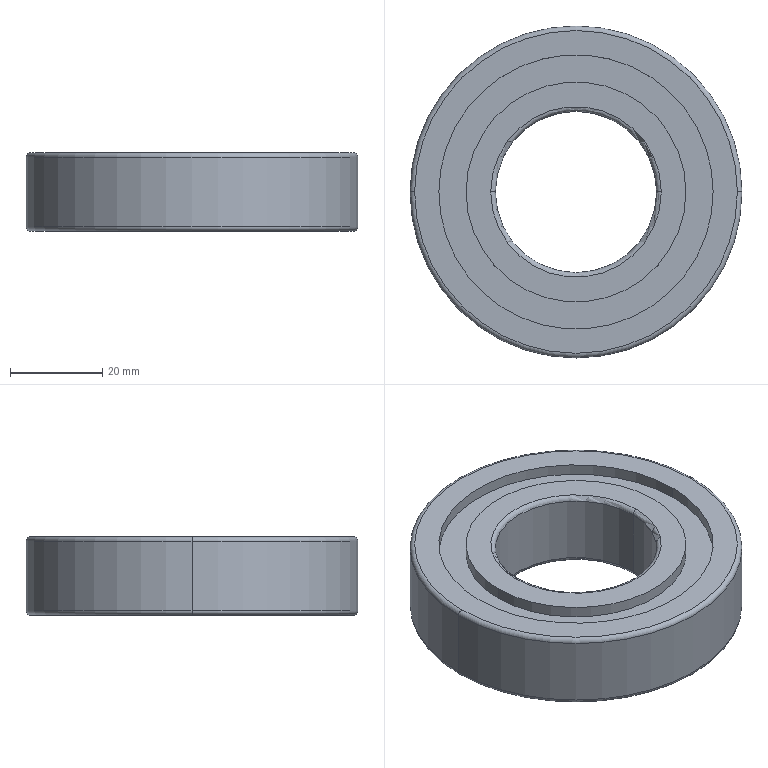Part | SolidWorks | features BaseBody 1 | 1 solid | 26 faces | box 72 x 72 x 17 mm | volume 47748 mm3 | cylinder 12 | torus 8 | plane 6 | commonest cylinder face diameters 47.7 x4 59.5 x4 35 x2 72 x2
STEP:
#1=CARTESIAN_POINT('',(358.083,269.388,35.922));
#2=VERTEX_POINT('',#1);
#3=CARTESIAN_POINT('',(323.083,269.388,35.922));
#4=VERTEX_POINT('',#3);
#5=CARTESIAN_POINT('',(340.583,269.388,35.922));
#6=DIRECTION('',(0.,0.,1.));
#7=DIRECTION('',(-1.,-0.000000008,0.));
#8=AXIS2_PLACEMENT_3D('',#5,#6,#7);
#9=CIRCLE('',#8,17.5);
#10=EDGE_CURVE('',#2,#4,#9,.T.);
#11=ORIENTED_EDGE('',*,*,#10,.T.);
#12=CARTESIAN_POINT('',(322.083,269.388,34.922));
#13=VERTEX_POINT('',#12);
#14=CARTESIAN_POINT('',(322.083,269.388,35.922));
#15=DIRECTION('',(-0.000000008,1.,0.));
#16=DIRECTION('',(-1.,-0.000000008,0.));
#17=AXIS2_PLACEMENT_3D('',#14,#15,#16);
#18=CIRCLE('',#17,1.);
#19=EDGE_CURVE('',#4,#13,#18,.T.);
#20=ORIENTED_EDGE('',*,*,#19,.T.);
#21=CARTESIAN_POINT('',(359.083,269.388,34.922));
#22=VERTEX_POINT('',#21);
#23=CARTESIAN_POINT('',(340.583,269.388,34.922));
#24=DIRECTION('',(0.,0.,1.));
#25=DIRECTION('',(-1.,-0.000000008,0.));
#26=AXIS2_PLACEMENT_3D('',#23,#24,#25);
#27=CIRCLE('',#26,18.5);
#28=EDGE_CURVE('',#22,#13,#27,.T.);
#29=ORIENTED_EDGE('',*,*,#28,.F.);
#30=CARTESIAN_POINT('',(359.083,269.388,35.922));
#31=DIRECTION('',(0.000000008,-1.,0.));
#32=DIRECTION('',(1.,0.000000008,0.));
#33=AXIS2_PLACEMENT_3D('',#30,#31,#32);
#34=CIRCLE('',#33,1.);
#35=EDGE_CURVE('',#2,#22,#34,.T.);
#36=ORIENTED_EDGE('',*,*,#35,.F.);
#37=EDGE_LOOP('',(#11,#20,#29,#36));
#38=FACE_OUTER_BOUND('',#37,.T.);
#39=CARTESIAN_POINT('',(340.583,269.388,35.922));
#40=DIRECTION('',(0.,0.,1.));
#41=DIRECTION('',(1.,0.000000008,0.));
#42=AXIS2_PLACEMENT_3D('',#39,#40,#41);
#43=TOROIDAL_SURFACE('',#42,18.5,1.);
#44=ADVANCED_FACE('',(#38),#43,.T.);
#45=CARTESIAN_POINT('',(340.583,269.388,35.922));
#46=DIRECTION('',(0.,0.,1.));
#47=DIRECTION('',(-1.,-0.000000008,0.));
#48=AXIS2_PLACEMENT_3D('',#45,#46,#47);
#49=CIRCLE('',#48,17.5);
#50=EDGE_CURVE('',#4,#2,#49,.T.);
#51=ORIENTED_EDGE('',*,*,#50,.F.);
#52=CARTESIAN_POINT('',(323.083,269.388,50.922));
#53=VERTEX_POINT('',#52);
#54=CARTESIAN_POINT('',(323.083,269.388,93.422));
#55=DIRECTION('',(0.,0.,1.));
#56=VECTOR('',#55,1000.);
#57=LINE('',#54,#56);
#58=EDGE_CURVE('',#4,#53,#57,.T.);
#59=ORIENTED_EDGE('',*,*,#58,.T.);
#60=CARTESIAN_POINT('',(358.083,269.388,50.922));
#61=VERTEX_POINT('',#60);
#62=CARTESIAN_POINT('',(340.583,269.388,50.922));
#63=DIRECTION('',(0.,0.,-1.));
#64=DIRECTION('',(1.,0.000000008,0.));
#65=AXIS2_PLACEMENT_3D('',#62,#63,#64);
#66=CIRCLE('',#65,17.5);
#67=EDGE_CURVE('',#61,#53,#66,.T.);
#68=ORIENTED_EDGE('',*,*,#67,.F.);
#69=CARTESIAN_POINT('',(358.083,269.388,93.422));
#70=DIRECTION('',(0.,0.,1.));
#71=VECTOR('',#70,1000.);
#72=LINE('',#69,#71);
#73=EDGE_CURVE('',#2,#61,#72,.T.);
#74=ORIENTED_EDGE('',*,*,#73,.F.);
#75=EDGE_LOOP('',(#51,#59,#68,#74));
#76=FACE_OUTER_BOUND('',#75,.T.);
#77=CARTESIAN_POINT('',(340.583,269.388,93.422));
#78=DIRECTION('',(0.,0.,1.));
#79=DIRECTION('',(1.,0.000000008,0.));
#80=AXIS2_PLACEMENT_3D('',#77,#78,#79);
#81=CYLINDRICAL_SURFACE('',#80,17.5);
#82=ADVANCED_FACE('',(#76),#81,.F.);
#83=CARTESIAN_POINT('',(322.083,269.388,51.922));
#84=VERTEX_POINT('',#83);
#85=CARTESIAN_POINT('',(359.083,269.388,51.922));
#86=VERTEX_POINT('',#85);
#87=CARTESIAN_POINT('',(340.583,269.388,51.922));
#88=DIRECTION('',(0.,0.,-1.));
#89=DIRECTION('',(-1.,-0.000000008,0.));
#90=AXIS2_PLACEMENT_3D('',#87,#88,#89);
#91=CIRCLE('',#90,18.5);
#92=EDGE_CURVE('',#84,#86,#91,.T.);
#93=ORIENTED_EDGE('',*,*,#92,.F.);
#94=CARTESIAN_POINT('',(322.083,269.388,50.922));
#95=DIRECTION('',(-0.000000008,1.,0.));
#96=DIRECTION('',(-1.,-0.000000008,0.));
#97=AXIS2_PLACEMENT_3D('',#94,#95,#96);
#98=CIRCLE('',#97,1.);
#99=EDGE_CURVE('',#84,#53,#98,.T.);
#100=ORIENTED_EDGE('',*,*,#99,.T.);
#101=CARTESIAN_POINT('',(340.583,269.388,50.922));
#102=DIRECTION('',(0.,0.,-1.));
#103=DIRECTION('',(1.,0.000000008,0.));
#104=AXIS2_PLACEMENT_3D('',#101,#102,#103);
#105=CIRCLE('',#104,17.5);
#106=EDGE_CURVE('',#53,#61,#105,.T.);
#107=ORIENTED_EDGE('',*,*,#106,.T.);
#108=CARTESIAN_POINT('',(359.083,269.388,50.922));
#109=DIRECTION('',(0.000000008,-1.,0.));
#110=DIRECTION('',(1.,0.000000008,0.));
#111=AXIS2_PLACEMENT_3D('',#108,#109,#110);
#112=CIRCLE('',#111,1.);
#113=EDGE_CURVE('',#86,#61,#112,.T.);
#114=ORIENTED_EDGE('',*,*,#113,.F.);
#115=EDGE_LOOP('',(#93,#100,#107,#114));
#116=FACE_OUTER_BOUND('',#115,.T.);
#117=CARTESIAN_POINT('',(340.583,269.388,50.922));
#118=DIRECTION('',(0.,0.,1.));
#119=DIRECTION('',(1.,0.000000008,0.));
#120=AXIS2_PLACEMENT_3D('',#117,#118,#119);
#121=TOROIDAL_SURFACE('',#120,18.5,1.);
#122=ADVANCED_FACE('',(#116),#121,.T.);
#123=CARTESIAN_POINT('',(316.733,269.388,49.422));
#124=VERTEX_POINT('',#123);
#125=CARTESIAN_POINT('',(364.433,269.388,49.422));
#126=VERTEX_POINT('',#125);
#127=CARTESIAN_POINT('',(340.583,269.388,49.422));
#128=DIRECTION('',(0.,0.,-1.));
#129=DIRECTION('',(-1.,-0.000000008,0.));
#130=AXIS2_PLACEMENT_3D('',#127,#128,#129);
#131=CIRCLE('',#130,23.85);
#132=EDGE_CURVE('',#124,#126,#131,.T.);
#133=ORIENTED_EDGE('',*,*,#132,.F.);
#134=CARTESIAN_POINT('',(316.733,269.388,51.922));
#135=VERTEX_POINT('',#134);
#136=CARTESIAN_POINT('',(316.733,269.388,51.922));
#137=DIRECTION('',(0.,0.,1.));
#138=VECTOR('',#137,1000.);
#139=LINE('',#136,#138);
#140=EDGE_CURVE('',#124,#135,#139,.T.);
#141=ORIENTED_EDGE('',*,*,#140,.T.);
#142=CARTESIAN_POINT('',(364.433,269.388,51.922));
#143=VERTEX_POINT('',#142);
#144=CARTESIAN_POINT('',(340.583,269.388,51.922));
#145=DIRECTION('',(0.,0.,1.));
#146=DIRECTION('',(-1.,-0.000000008,0.));
#147=AXIS2_PLACEMENT_3D('',#144,#145,#146);
#148=CIRCLE('',#147,23.85);
#149=EDGE_CURVE('',#143,#135,#148,.T.);
#150=ORIENTED_EDGE('',*,*,#149,.F.);
#151=CARTESIAN_POINT('',(364.433,269.388,51.922));
#152=DIRECTION('',(0.,0.,1.));
#153=VECTOR('',#152,1000.);
#154=LINE('',#151,#153);
#155=EDGE_CURVE('',#126,#143,#154,.T.);
#156=ORIENTED_EDGE('',*,*,#155,.F.);
#157=EDGE_LOOP('',(#133,#141,#150,#156));
#158=FACE_OUTER_BOUND('',#157,.T.);
#159=CARTESIAN_POINT('',(340.583,269.388,51.922));
#160=DIRECTION('',(0.,0.,1.));
#161=DIRECTION('',(1.,0.000000008,0.));
#162=AXIS2_PLACEMENT_3D('',#159,#160,#161);
#163=CYLINDRICAL_SURFACE('',#162,23.85);
#164=ADVANCED_FACE('',(#158),#163,.T.);
#165=CARTESIAN_POINT('',(310.833,269.388,49.422));
#166=VERTEX_POINT('',#165);
#167=CARTESIAN_POINT('',(370.333,269.388,49.422));
#168=VERTEX_POINT('',#167);
#169=CARTESIAN_POINT('',(340.583,269.388,49.422));
#170=DIRECTION('',(0.,0.,1.));
#171=DIRECTION('',(-1.,-0.000000008,0.));
#172=AXIS2_PLACEMENT_3D('',#169,#170,#171);
#173=CIRCLE('',#172,29.75);
#174=EDGE_CURVE('',#166,#168,#173,.T.);
#175=ORIENTED_EDGE('',*,*,#174,.F.);
#176=CARTESIAN_POINT('',(310.833,269.388,51.922));
#177=VERTEX_POINT('',#176);
#178=CARTESIAN_POINT('',(310.833,269.388,51.922));
#179=DIRECTION('',(0.,0.,1.));
#180=VECTOR('',#179,1000.);
#181=LINE('',#178,#180);
#182=EDGE_CURVE('',#166,#177,#181,.T.);
#183=ORIENTED_EDGE('',*,*,#182,.T.);
#184=CARTESIAN_POINT('',(370.333,269.388,51.922));
#185=VERTEX_POINT('',#184);
#186=CARTESIAN_POINT('',(340.583,269.388,51.922));
#187=DIRECTION('',(0.,0.,-1.));
#188=DIRECTION('',(-1.,-0.000000008,0.));
#189=AXIS2_PLACEMENT_3D('',#186,#187,#188);
#190=CIRCLE('',#189,29.75);
#191=EDGE_CURVE('',#185,#177,#190,.T.);
#192=ORIENTED_EDGE('',*,*,#191,.F.);
#193=CARTESIAN_POINT('',(370.333,269.388,51.922));
#194=DIRECTION('',(0.,0.,1.));
#195=VECTOR('',#194,1000.);
#196=LINE('',#193,#195);
#197=EDGE_CURVE('',#168,#185,#196,.T.);
#198=ORIENTED_EDGE('',*,*,#197,.F.);
#199=EDGE_LOOP('',(#175,#183,#192,#198));
#200=FACE_OUTER_BOUND('',#199,.T.);
#201=CARTESIAN_POINT('',(340.583,269.388,51.922));
#202=DIRECTION('',(0.,0.,1.));
#203=DIRECTION('',(1.,0.000000008,0.));
#204=AXIS2_PLACEMENT_3D('',#201,#202,#203);
#205=CYLINDRICAL_SURFACE('',#204,29.75);
#206=ADVANCED_FACE('',(#200),#205,.F.);
#207=CARTESIAN_POINT('',(376.583,269.388,50.922));
#208=VERTEX_POINT('',#207);
#209=CARTESIAN_POINT('',(304.583,269.388,50.922));
#210=VERTEX_POINT('',#209);
#211=CARTESIAN_POINT('',(340.583,269.388,50.922));
#212=DIRECTION('',(0.,0.,1.));
#213=DIRECTION('',(-1.,-0.000000008,0.));
#214=AXIS2_PLACEMENT_3D('',#211,#212,#213);
#215=CIRCLE('',#214,36.);
#216=EDGE_CURVE('',#208,#210,#215,.T.);
#217=ORIENTED_EDGE('',*,*,#216,.T.);
#218=CARTESIAN_POINT('',(305.583,269.388,51.922));
#219=VERTEX_POINT('',#218);
#220=CARTESIAN_POINT('',(305.583,269.388,50.922));
#221=DIRECTION('',(-0.000000008,1.,0.));
#222=DIRECTION('',(-1.,-0.000000008,0.));
#223=AXIS2_PLACEMENT_3D('',#220,#221,#222);
#224=CIRCLE('',#223,1.);
#225=EDGE_CURVE('',#210,#219,#224,.T.);
#226=ORIENTED_EDGE('',*,*,#225,.T.);
#227=CARTESIAN_POINT('',(375.583,269.388,51.922));
#228=VERTEX_POINT('',#227);
#229=CARTESIAN_POINT('',(340.583,269.388,51.922));
#230=DIRECTION('',(0.,0.,1.));
#231=DIRECTION('',(-1.,-0.000000008,0.));
#232=AXIS2_PLACEMENT_3D('',#229,#230,#231);
#233=CIRCLE('',#232,35.);
#234=EDGE_CURVE('',#228,#219,#233,.T.);
#235=ORIENTED_EDGE('',*,*,#234,.F.);
#236=CARTESIAN_POINT('',(375.583,269.388,50.922));
#237=DIRECTION('',(0.000000008,-1.,0.));
#238=DIRECTION('',(1.,0.000000008,0.));
#239=AXIS2_PLACEMENT_3D('',#236,#237,#238);
#240=CIRCLE('',#239,1.);
#241=EDGE_CURVE('',#208,#228,#240,.T.);
#242=ORIENTED_EDGE('',*,*,#241,.F.);
#243=EDGE_LOOP('',(#217,#226,#235,#242));
#244=FACE_OUTER_BOUND('',#243,.T.);
#245=CARTESIAN_POINT('',(340.583,269.388,50.922));
#246=DIRECTION('',(0.,0.,1.));
#247=DIRECTION('',(1.,0.000000008,0.));
#248=AXIS2_PLACEMENT_3D('',#245,#246,#247);
#249=TOROIDAL_SURFACE('',#248,35.,1.);
#250=ADVANCED_FACE('',(#244),#249,.T.);
#251=CARTESIAN_POINT('',(304.583,269.388,35.922));
#252=VERTEX_POINT('',#251);
#253=CARTESIAN_POINT('',(376.583,269.388,35.922));
#254=VERTEX_POINT('',#253);
#255=CARTESIAN_POINT('',(340.583,269.388,35.922));
#256=DIRECTION('',(0.,0.,-1.));
#257=DIRECTION('',(1.,0.000000008,0.));
#258=AXIS2_PLACEMENT_3D('',#255,#256,#257);
#259=CIRCLE('',#258,36.);
#260=EDGE_CURVE('',#252,#254,#259,.T.);
#261=ORIENTED_EDGE('',*,*,#260,.F.);
#262=CARTESIAN_POINT('',(304.583,269.388,51.922));
#263=DIRECTION('',(0.,0.,1.));
#264=VECTOR('',#263,1000.);
#265=LINE('',#262,#264);
#266=EDGE_CURVE('',#252,#210,#265,.T.);
#267=ORIENTED_EDGE('',*,*,#266,.T.);
#268=ORIENTED_EDGE('',*,*,#216,.F.);
#269=CARTESIAN_POINT('',(376.583,269.388,51.922));
#270=DIRECTION('',(0.,0.,1.));
#271=VECTOR('',#270,1000.);
#272=LINE('',#269,#271);
#273=EDGE_CURVE('',#254,#208,#272,.T.);
#274=ORIENTED_EDGE('',*,*,#273,.F.);
#275=EDGE_LOOP('',(#261,#267,#268,#274));
#276=FACE_OUTER_BOUND('',#275,.T.);
#277=CARTESIAN_POINT('',(340.583,269.388,51.922));
#278=DIRECTION('',(0.,0.,1.));
#279=DIRECTION('',(1.,0.000000008,0.));
#280=AXIS2_PLACEMENT_3D('',#277,#278,#279);
#281=CYLINDRICAL_SURFACE('',#280,36.);
#282=ADVANCED_FACE('',(#276),#281,.T.);
#283=CARTESIAN_POINT('',(305.583,269.388,34.922));
#284=VERTEX_POINT('',#283);
#285=CARTESIAN_POINT('',(375.583,269.388,34.922));
#286=VERTEX_POINT('',#285);
#287=CARTESIAN_POINT('',(340.583,269.388,34.922));
#288=DIRECTION('',(0.,0.,-1.));
#289=DIRECTION('',(1.,0.000000008,0.));
#290=AXIS2_PLACEMENT_3D('',#287,#288,#289);
#291=CIRCLE('',#290,35.);
#292=EDGE_CURVE('',#284,#286,#291,.T.);
#293=ORIENTED_EDGE('',*,*,#292,.F.);
#294=CARTESIAN_POINT('',(305.583,269.388,35.922));
#295=DIRECTION('',(-0.000000008,1.,0.));
#296=DIRECTION('',(-1.,-0.000000008,0.));
#297=AXIS2_PLACEMENT_3D('',#294,#295,#296);
#298=CIRCLE('',#297,1.);
#299=EDGE_CURVE('',#284,#252,#298,.T.);
#300=ORIENTED_EDGE('',*,*,#299,.T.);
#301=ORIENTED_EDGE('',*,*,#260,.T.);
#302=CARTESIAN_POINT('',(375.583,269.388,35.922));
#303=DIRECTION('',(0.000000008,-1.,0.));
#304=DIRECTION('',(1.,0.000000008,0.));
#305=AXIS2_PLACEMENT_3D('',#302,#303,#304);
#306=CIRCLE('',#305,1.);
#307=EDGE_CURVE('',#286,#254,#306,.T.);
#308=ORIENTED_EDGE('',*,*,#307,.F.);
#309=EDGE_LOOP('',(#293,#300,#301,#308));
#310=FACE_OUTER_BOUND('',#309,.T.);
#311=CARTESIAN_POINT('',(340.583,269.388,35.922));
#312=DIRECTION('',(0.,0.,1.));
#313=DIRECTION('',(1.,0.000000008,0.));
#314=AXIS2_PLACEMENT_3D('',#311,#312,#313);
#315=TOROIDAL_SURFACE('',#314,35.,1.);
#316=ADVANCED_FACE('',(#310),#315,.T.);
#317=CARTESIAN_POINT('',(310.833,269.388,34.922));
#318=VERTEX_POINT('',#317);
#319=CARTESIAN_POINT('',(370.333,269.388,34.922));
#320=VERTEX_POINT('',#319);
#321=CARTESIAN_POINT('',(340.583,269.388,34.922));
#322=DIRECTION('',(0.,0.,1.));
#323=DIRECTION('',(-1.,-0.000000008,0.));
#324=AXIS2_PLACEMENT_3D('',#321,#322,#323);
#325=CIRCLE('',#324,29.75);
#326=EDGE_CURVE('',#318,#320,#325,.T.);
#327=ORIENTED_EDGE('',*,*,#326,.F.);
#328=CARTESIAN_POINT('',(310.833,269.388,37.422));
#329=VERTEX_POINT('',#328);
#330=CARTESIAN_POINT('',(310.833,269.388,51.922));
#331=DIRECTION('',(0.,0.,1.));
#332=VECTOR('',#331,1000.);
#333=LINE('',#330,#332);
#334=EDGE_CURVE('',#318,#329,#333,.T.);
#335=ORIENTED_EDGE('',*,*,#334,.T.);
#336=CARTESIAN_POINT('',(370.333,269.388,37.422));
#337=VERTEX_POINT('',#336);
#338=CARTESIAN_POINT('',(340.583,269.388,37.422));
#339=DIRECTION('',(0.,0.,-1.));
#340=DIRECTION('',(-1.,-0.000000008,0.));
#341=AXIS2_PLACEMENT_3D('',#338,#339,#340);
#342=CIRCLE('',#341,29.75);
#343=EDGE_CURVE('',#337,#329,#342,.T.);
#344=ORIENTED_EDGE('',*,*,#343,.F.);
#345=CARTESIAN_POINT('',(370.333,269.388,51.922));
#346=DIRECTION('',(0.,0.,1.));
#347=VECTOR('',#346,1000.);
#348=LINE('',#345,#347);
#349=EDGE_CURVE('',#320,#337,#348,.T.);
#350=ORIENTED_EDGE('',*,*,#349,.F.);
#351=EDGE_LOOP('',(#327,#335,#344,#350));
#352=FACE_OUTER_BOUND('',#351,.T.);
#353=CARTESIAN_POINT('',(340.583,269.388,51.922));
#354=DIRECTION('',(0.,0.,1.));
#355=DIRECTION('',(1.,0.000000008,0.));
#356=AXIS2_PLACEMENT_3D('',#353,#354,#355);
#357=CYLINDRICAL_SURFACE('',#356,29.75);
#358=ADVANCED_FACE('',(#352),#357,.F.);
#359=CARTESIAN_POINT('',(316.733,269.388,34.922));
#360=VERTEX_POINT('',#359);
#361=CARTESIAN_POINT('',(364.433,269.388,34.922));
#362=VERTEX_POINT('',#361);
#363=CARTESIAN_POINT('',(340.583,269.388,34.922));
#364=DIRECTION('',(0.,0.,-1.));
#365=DIRECTION('',(-1.,-0.000000008,0.));
#366=AXIS2_PLACEMENT_3D('',#363,#364,#365);
#367=CIRCLE('',#366,23.85);
#368=EDGE_CURVE('',#360,#362,#367,.T.);
#369=ORIENTED_EDGE('',*,*,#368,.F.);
#370=CARTESIAN_POINT('',(316.733,269.388,37.422));
#371=VERTEX_POINT('',#370);
#372=CARTESIAN_POINT('',(316.733,269.388,51.922));
#373=DIRECTION('',(0.,0.,1.));
#374=VECTOR('',#373,1000.);
#375=LINE('',#372,#374);
#376=EDGE_CURVE('',#360,#371,#375,.T.);
#377=ORIENTED_EDGE('',*,*,#376,.T.);
#378=CARTESIAN_POINT('',(364.433,269.388,37.422));
#379=VERTEX_POINT('',#378);
#380=CARTESIAN_POINT('',(340.583,269.388,37.422));
#381=DIRECTION('',(0.,0.,1.));
#382=DIRECTION('',(-1.,-0.000000008,0.));
#383=AXIS2_PLACEMENT_3D('',#380,#381,#382);
#384=CIRCLE('',#383,23.85);
#385=EDGE_CURVE('',#379,#371,#384,.T.);
#386=ORIENTED_EDGE('',*,*,#385,.F.);
#387=CARTESIAN_POINT('',(364.433,269.388,51.922));
#388=DIRECTION('',(0.,0.,1.));
#389=VECTOR('',#388,1000.);
#390=LINE('',#387,#389);
#391=EDGE_CURVE('',#362,#379,#390,.T.);
#392=ORIENTED_EDGE('',*,*,#391,.F.);
#393=EDGE_LOOP('',(#369,#377,#386,#392));
#394=FACE_OUTER_BOUND('',#393,.T.);
#395=CARTESIAN_POINT('',(340.583,269.388,51.922));
#396=DIRECTION('',(0.,0.,1.));
#397=DIRECTION('',(1.,0.000000008,0.));
#398=AXIS2_PLACEMENT_3D('',#395,#396,#397);
#399=CYLINDRICAL_SURFACE('',#398,23.85);
#400=ADVANCED_FACE('',(#394),#399,.T.);
#401=ORIENTED_EDGE('',*,*,#376,.F.);
#402=CARTESIAN_POINT('',(340.583,269.388,34.922));
#403=DIRECTION('',(0.,0.,-1.));
#404=DIRECTION('',(-1.,-0.000000008,0.));
#405=AXIS2_PLACEMENT_3D('',#402,#403,#404);
#406=CIRCLE('',#405,23.85);
#407=EDGE_CURVE('',#362,#360,#406,.T.);
#408=ORIENTED_EDGE('',*,*,#407,.F.);
#409=ORIENTED_EDGE('',*,*,#391,.T.);
#410=CARTESIAN_POINT('',(340.583,269.388,37.422));
#411=DIRECTION('',(0.,0.,1.));
#412=DIRECTION('',(-1.,-0.000000008,0.));
#413=AXIS2_PLACEMENT_3D('',#410,#411,#412);
#414=CIRCLE('',#413,23.85);
#415=EDGE_CURVE('',#371,#379,#414,.T.);
#416=ORIENTED_EDGE('',*,*,#415,.F.);
#417=EDGE_LOOP('',(#401,#408,#409,#416));
#418=FACE_OUTER_BOUND('',#417,.T.);
#419=CARTESIAN_POINT('',(340.583,269.388,51.922));
#420=DIRECTION('',(0.,0.,1.));
#421=DIRECTION('',(1.,0.000000008,0.));
#422=AXIS2_PLACEMENT_3D('',#419,#420,#421);
#423=CYLINDRICAL_SURFACE('',#422,23.85);
#424=ADVANCED_FACE('',(#418),#423,.T.);
#425=ORIENTED_EDGE('',*,*,#385,.T.);
#426=ORIENTED_EDGE('',*,*,#415,.T.);
#427=EDGE_LOOP('',(#425,#426));
#428=FACE_BOUND('',#427,.T.);
#429=ORIENTED_EDGE('',*,*,#343,.T.);
#430=CARTESIAN_POINT('',(340.583,269.388,37.422));
#431=DIRECTION('',(0.,0.,-1.));
#432=DIRECTION('',(-1.,-0.000000008,0.));
#433=AXIS2_PLACEMENT_3D('',#430,#431,#432);
#434=CIRCLE('',#433,29.75);
#435=EDGE_CURVE('',#329,#337,#434,.T.);
#436=ORIENTED_EDGE('',*,*,#435,.T.);
#437=EDGE_LOOP('',(#429,#436));
#438=FACE_OUTER_BOUND('',#437,.T.);
#439=CARTESIAN_POINT('',(340.583,293.238,37.422));
#440=DIRECTION('',(0.,0.,1.));
#441=DIRECTION('',(0.,-1.,0.));
#442=AXIS2_PLACEMENT_3D('',#439,#440,#441);
#443=PLANE('',#442);
#444=ADVANCED_FACE('',(#428,#438),#443,.F.);
#445=ORIENTED_EDGE('',*,*,#334,.F.);
#446=CARTESIAN_POINT('',(340.583,269.388,34.922));
#447=DIRECTION('',(0.,0.,1.));
#448=DIRECTION('',(-1.,-0.000000008,0.));
#449=AXIS2_PLACEMENT_3D('',#446,#447,#448);
#450=CIRCLE('',#449,29.75);
#451=EDGE_CURVE('',#320,#318,#450,.T.);
#452=ORIENTED_EDGE('',*,*,#451,.F.);
#453=ORIENTED_EDGE('',*,*,#349,.T.);
#454=ORIENTED_EDGE('',*,*,#435,.F.);
#455=EDGE_LOOP('',(#445,#452,#453,#454));
#456=FACE_OUTER_BOUND('',#455,.T.);
#457=CARTESIAN_POINT('',(340.583,269.388,51.922));
#458=DIRECTION('',(0.,0.,1.));
#459=DIRECTION('',(1.,0.000000008,0.));
#460=AXIS2_PLACEMENT_3D('',#457,#458,#459);
#461=CYLINDRICAL_SURFACE('',#460,29.75);
#462=ADVANCED_FACE('',(#456),#461,.F.);
#463=ORIENTED_EDGE('',*,*,#451,.T.);
#464=ORIENTED_EDGE('',*,*,#326,.T.);
#465=EDGE_LOOP('',(#463,#464));
#466=FACE_BOUND('',#465,.T.);
#467=CARTESIAN_POINT('',(340.583,269.388,34.922));
#468=DIRECTION('',(0.,0.,-1.));
#469=DIRECTION('',(1.,0.000000008,0.));
#470=AXIS2_PLACEMENT_3D('',#467,#468,#469);
#471=CIRCLE('',#470,35.);
#472=EDGE_CURVE('',#286,#284,#471,.T.);
#473=ORIENTED_EDGE('',*,*,#472,.T.);
#474=ORIENTED_EDGE('',*,*,#292,.T.);
#475=EDGE_LOOP('',(#473,#474));
#476=FACE_OUTER_BOUND('',#475,.T.);
#477=CARTESIAN_POINT('',(340.583,299.138,34.922));
#478=DIRECTION('',(0.,0.,1.));
#479=DIRECTION('',(0.,-1.,0.));
#480=AXIS2_PLACEMENT_3D('',#477,#478,#479);
#481=PLANE('',#480);
#482=ADVANCED_FACE('',(#466,#476),#481,.F.);
#483=ORIENTED_EDGE('',*,*,#299,.F.);
#484=ORIENTED_EDGE('',*,*,#472,.F.);
#485=ORIENTED_EDGE('',*,*,#307,.T.);
#486=CARTESIAN_POINT('',(340.583,269.388,35.922));
#487=DIRECTION('',(0.,0.,-1.));
#488=DIRECTION('',(1.,0.000000008,0.));
#489=AXIS2_PLACEMENT_3D('',#486,#487,#488);
#490=CIRCLE('',#489,36.);
#491=EDGE_CURVE('',#254,#252,#490,.T.);
#492=ORIENTED_EDGE('',*,*,#491,.T.);
#493=EDGE_LOOP('',(#483,#484,#485,#492));
#494=FACE_OUTER_BOUND('',#493,.T.);
#495=CARTESIAN_POINT('',(340.583,269.388,35.922));
#496=DIRECTION('',(0.,0.,1.));
#497=DIRECTION('',(1.,0.000000008,0.));
#498=AXIS2_PLACEMENT_3D('',#495,#496,#497);
#499=TOROIDAL_SURFACE('',#498,35.,1.);
#500=ADVANCED_FACE('',(#494),#499,.T.);
#501=ORIENTED_EDGE('',*,*,#266,.F.);
#502=ORIENTED_EDGE('',*,*,#491,.F.);
#503=ORIENTED_EDGE('',*,*,#273,.T.);
#504=CARTESIAN_POINT('',(340.583,269.388,50.922));
#505=DIRECTION('',(0.,0.,1.));
#506=DIRECTION('',(-1.,-0.000000008,0.));
#507=AXIS2_PLACEMENT_3D('',#504,#505,#506);
#508=CIRCLE('',#507,36.);
#509=EDGE_CURVE('',#210,#208,#508,.T.);
#510=ORIENTED_EDGE('',*,*,#509,.F.);
#511=EDGE_LOOP('',(#501,#502,#503,#510));
#512=FACE_OUTER_BOUND('',#511,.T.);
#513=CARTESIAN_POINT('',(340.583,269.388,51.922));
#514=DIRECTION('',(0.,0.,1.));
#515=DIRECTION('',(1.,0.000000008,0.));
#516=AXIS2_PLACEMENT_3D('',#513,#514,#515);
#517=CYLINDRICAL_SURFACE('',#516,36.);
#518=ADVANCED_FACE('',(#512),#517,.T.);
#519=ORIENTED_EDGE('',*,*,#225,.F.);
#520=ORIENTED_EDGE('',*,*,#509,.T.);
#521=ORIENTED_EDGE('',*,*,#241,.T.);
#522=CARTESIAN_POINT('',(340.583,269.388,51.922));
#523=DIRECTION('',(0.,0.,1.));
#524=DIRECTION('',(-1.,-0.000000008,0.));
#525=AXIS2_PLACEMENT_3D('',#522,#523,#524);
#526=CIRCLE('',#525,35.);
#527=EDGE_CURVE('',#219,#228,#526,.T.);
#528=ORIENTED_EDGE('',*,*,#527,.F.);
#529=EDGE_LOOP('',(#519,#520,#521,#528));
#530=FACE_OUTER_BOUND('',#529,.T.);
#531=CARTESIAN_POINT('',(340.583,269.388,50.922));
#532=DIRECTION('',(0.,0.,1.));
#533=DIRECTION('',(1.,0.000000008,0.));
#534=AXIS2_PLACEMENT_3D('',#531,#532,#533);
#535=TOROIDAL_SURFACE('',#534,35.,1.);
#536=ADVANCED_FACE('',(#530),#535,.T.);
#537=ORIENTED_EDGE('',*,*,#191,.T.);
#538=CARTESIAN_POINT('',(340.583,269.388,51.922));
#539=DIRECTION('',(0.,0.,-1.));
#540=DIRECTION('',(-1.,-0.000000008,0.));
#541=AXIS2_PLACEMENT_3D('',#538,#539,#540);
#542=CIRCLE('',#541,29.75);
#543=EDGE_CURVE('',#177,#185,#542,.T.);
#544=ORIENTED_EDGE('',*,*,#543,.T.);
#545=EDGE_LOOP('',(#537,#544));
#546=FACE_BOUND('',#545,.T.);
#547=ORIENTED_EDGE('',*,*,#234,.T.);
#548=ORIENTED_EDGE('',*,*,#527,.T.);
#549=EDGE_LOOP('',(#547,#548));
#550=FACE_OUTER_BOUND('',#549,.T.);
#551=CARTESIAN_POINT('',(340.583,304.388,51.922));
#552=DIRECTION('',(0.,0.,-1.));
#553=DIRECTION('',(-1.,0.,0.));
#554=AXIS2_PLACEMENT_3D('',#551,#552,#553);
#555=PLANE('',#554);
#556=ADVANCED_FACE('',(#546,#550),#555,.F.);
#557=ORIENTED_EDGE('',*,*,#182,.F.);
#558=CARTESIAN_POINT('',(340.583,269.388,49.422));
#559=DIRECTION('',(0.,0.,1.));
#560=DIRECTION('',(-1.,-0.000000008,0.));
#561=AXIS2_PLACEMENT_3D('',#558,#559,#560);
#562=CIRCLE('',#561,29.75);
#563=EDGE_CURVE('',#168,#166,#562,.T.);
#564=ORIENTED_EDGE('',*,*,#563,.F.);
#565=ORIENTED_EDGE('',*,*,#197,.T.);
#566=ORIENTED_EDGE('',*,*,#543,.F.);
#567=EDGE_LOOP('',(#557,#564,#565,#566));
#568=FACE_OUTER_BOUND('',#567,.T.);
#569=CARTESIAN_POINT('',(340.583,269.388,51.922));
#570=DIRECTION('',(0.,0.,1.));
#571=DIRECTION('',(1.,0.000000008,0.));
#572=AXIS2_PLACEMENT_3D('',#569,#570,#571);
#573=CYLINDRICAL_SURFACE('',#572,29.75);
#574=ADVANCED_FACE('',(#568),#573,.F.);
#575=CARTESIAN_POINT('',(340.583,269.388,49.422));
#576=DIRECTION('',(0.,0.,-1.));
#577=DIRECTION('',(-1.,-0.000000008,0.));
#578=AXIS2_PLACEMENT_3D('',#575,#576,#577);
#579=CIRCLE('',#578,23.85);
#580=EDGE_CURVE('',#126,#124,#579,.T.);
#581=ORIENTED_EDGE('',*,*,#580,.T.);
#582=ORIENTED_EDGE('',*,*,#132,.T.);
#583=EDGE_LOOP('',(#581,#582));
#584=FACE_BOUND('',#583,.T.);
#585=ORIENTED_EDGE('',*,*,#563,.T.);
#586=ORIENTED_EDGE('',*,*,#174,.T.);
#587=EDGE_LOOP('',(#585,#586));
#588=FACE_OUTER_BOUND('',#587,.T.);
#589=CARTESIAN_POINT('',(340.583,299.138,49.422));
#590=DIRECTION('',(0.,0.,-1.));
#591=DIRECTION('',(-1.,0.,0.));
#592=AXIS2_PLACEMENT_3D('',#589,#590,#591);
#593=PLANE('',#592);
#594=ADVANCED_FACE('',(#584,#588),#593,.F.);
#595=ORIENTED_EDGE('',*,*,#140,.F.);
#596=ORIENTED_EDGE('',*,*,#580,.F.);
#597=ORIENTED_EDGE('',*,*,#155,.T.);
#598=CARTESIAN_POINT('',(340.583,269.388,51.922));
#599=DIRECTION('',(0.,0.,1.));
#600=DIRECTION('',(-1.,-0.000000008,0.));
#601=AXIS2_PLACEMENT_3D('',#598,#599,#600);
#602=CIRCLE('',#601,23.85);
#603=EDGE_CURVE('',#135,#143,#602,.T.);
#604=ORIENTED_EDGE('',*,*,#603,.F.);
#605=EDGE_LOOP('',(#595,#596,#597,#604));
#606=FACE_OUTER_BOUND('',#605,.T.);
#607=CARTESIAN_POINT('',(340.583,269.388,51.922));
#608=DIRECTION('',(0.,0.,1.));
#609=DIRECTION('',(1.,0.000000008,0.));
#610=AXIS2_PLACEMENT_3D('',#607,#608,#609);
#611=CYLINDRICAL_SURFACE('',#610,23.85);
#612=ADVANCED_FACE('',(#606),#611,.T.);
#613=CARTESIAN_POINT('',(340.583,269.388,51.922));
#614=DIRECTION('',(0.,0.,-1.));
#615=DIRECTION('',(-1.,-0.000000008,0.));
#616=AXIS2_PLACEMENT_3D('',#613,#614,#615);
#617=CIRCLE('',#616,18.5);
#618=EDGE_CURVE('',#86,#84,#617,.T.);
#619=ORIENTED_EDGE('',*,*,#618,.T.);
#620=ORIENTED_EDGE('',*,*,#92,.T.);
#621=EDGE_LOOP('',(#619,#620));
#622=FACE_BOUND('',#621,.T.);
#623=ORIENTED_EDGE('',*,*,#149,.T.);
#624=ORIENTED_EDGE('',*,*,#603,.T.);
#625=EDGE_LOOP('',(#623,#624));
#626=FACE_OUTER_BOUND('',#625,.T.);
#627=CARTESIAN_POINT('',(340.583,293.238,51.922));
#628=DIRECTION('',(0.,0.,-1.));
#629=DIRECTION('',(-1.,0.,0.));
#630=AXIS2_PLACEMENT_3D('',#627,#628,#629);
#631=PLANE('',#630);
#632=ADVANCED_FACE('',(#622,#626),#631,.F.);
#633=ORIENTED_EDGE('',*,*,#99,.F.);
#634=ORIENTED_EDGE('',*,*,#618,.F.);
#635=ORIENTED_EDGE('',*,*,#113,.T.);
#636=ORIENTED_EDGE('',*,*,#67,.T.);
#637=EDGE_LOOP('',(#633,#634,#635,#636));
#638=FACE_OUTER_BOUND('',#637,.T.);
#639=CARTESIAN_POINT('',(340.583,269.388,50.922));
#640=DIRECTION('',(0.,0.,1.));
#641=DIRECTION('',(1.,0.000000008,0.));
#642=AXIS2_PLACEMENT_3D('',#639,#640,#641);
#643=TOROIDAL_SURFACE('',#642,18.5,1.);
#644=ADVANCED_FACE('',(#638),#643,.T.);
#645=ORIENTED_EDGE('',*,*,#58,.F.);
#646=ORIENTED_EDGE('',*,*,#10,.F.);
#647=ORIENTED_EDGE('',*,*,#73,.T.);
#648=ORIENTED_EDGE('',*,*,#106,.F.);
#649=EDGE_LOOP('',(#645,#646,#647,#648));
#650=FACE_OUTER_BOUND('',#649,.T.);
#651=CARTESIAN_POINT('',(340.583,269.388,93.422));
#652=DIRECTION('',(0.,0.,1.));
#653=DIRECTION('',(1.,0.000000008,0.));
#654=AXIS2_PLACEMENT_3D('',#651,#652,#653);
#655=CYLINDRICAL_SURFACE('',#654,17.5);
#656=ADVANCED_FACE('',(#650),#655,.F.);
#657=ORIENTED_EDGE('',*,*,#19,.F.);
#658=ORIENTED_EDGE('',*,*,#50,.T.);
#659=ORIENTED_EDGE('',*,*,#35,.T.);
#660=CARTESIAN_POINT('',(340.583,269.388,34.922));
#661=DIRECTION('',(0.,0.,1.));
#662=DIRECTION('',(-1.,-0.000000008,0.));
#663=AXIS2_PLACEMENT_3D('',#660,#661,#662);
#664=CIRCLE('',#663,18.5);
#665=EDGE_CURVE('',#13,#22,#664,.T.);
#666=ORIENTED_EDGE('',*,*,#665,.F.);
#667=EDGE_LOOP('',(#657,#658,#659,#666));
#668=FACE_OUTER_BOUND('',#667,.T.);
#669=CARTESIAN_POINT('',(340.583,269.388,35.922));
#670=DIRECTION('',(0.,0.,1.));
#671=DIRECTION('',(1.,0.000000008,0.));
#672=AXIS2_PLACEMENT_3D('',#669,#670,#671);
#673=TOROIDAL_SURFACE('',#672,18.5,1.);
#674=ADVANCED_FACE('',(#668),#673,.T.);
#675=ORIENTED_EDGE('',*,*,#28,.T.);
#676=ORIENTED_EDGE('',*,*,#665,.T.);
#677=EDGE_LOOP('',(#675,#676));
#678=FACE_BOUND('',#677,.T.);
#679=ORIENTED_EDGE('',*,*,#407,.T.);
#680=ORIENTED_EDGE('',*,*,#368,.T.);
#681=EDGE_LOOP('',(#679,#680));
#682=FACE_OUTER_BOUND('',#681,.T.);
#683=CARTESIAN_POINT('',(340.583,269.388,34.922));
#684=DIRECTION('',(0.,0.,1.));
#685=DIRECTION('',(0.,-1.,0.));
#686=AXIS2_PLACEMENT_3D('',#683,#684,#685);
#687=PLANE('',#686);
#688=ADVANCED_FACE('',(#678,#682),#687,.F.);
#689=CLOSED_SHELL('',(#44,#82,#122,#164,#206,#250,#282,#316,#358,#400,#424,#444,#462,#482,#500,#518,#536,#556,#574,#594,#612,#632,#644,#656,#674,#688));
#690=MANIFOLD_SOLID_BREP('',#689);
#691=CARTESIAN_POINT('',(0.,0.,0.));
#692=DIRECTION('',(0.,0.,1.));
#693=DIRECTION('',(1.,0.,0.));
#694=AXIS2_PLACEMENT_3D('',#691,#692,#693);
#695=(LENGTH_UNIT()NAMED_UNIT(*)SI_UNIT(.MILLI.,.METRE.));
#696=UNCERTAINTY_MEASURE_WITH_UNIT(LENGTH_MEASURE(0.00001),#695,'','');
#697=(NAMED_UNIT(*)PLANE_ANGLE_UNIT()SI_UNIT($,.RADIAN.));
#698=(NAMED_UNIT(*)SI_UNIT($,.STERADIAN.)SOLID_ANGLE_UNIT());
#699=(GEOMETRIC_REPRESENTATION_CONTEXT(3)GLOBAL_UNCERTAINTY_ASSIGNED_CONTEXT((#696))GLOBAL_UNIT_ASSIGNED_CONTEXT((#695,#697,#698))REPRESENTATION_CONTEXT('',''));
#700=ADVANCED_BREP_SHAPE_REPRESENTATION('',(#690,#694),#699);